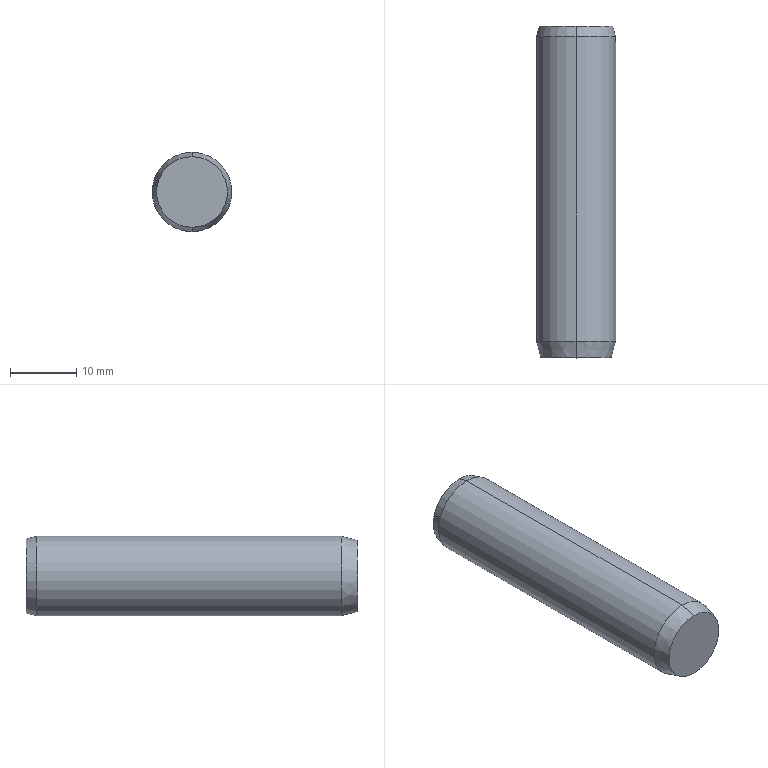Part | SolidWorks | features Chamfer 2, Extrusion 1, HoleWzd 1 | 1 solid | 12 faces | box 12 x 50 x 12 mm | volume 5242 mm3 | cone 6 | cylinder 4 | plane 2 | commonest cylinder face diameters 4.8 x2 12 x2
STEP:
#1=CARTESIAN_POINT('',(0.,-25.,-5.33));
#2=VERTEX_POINT('',#1);
#3=CARTESIAN_POINT('',(0.,-25.,5.33));
#4=VERTEX_POINT('',#3);
#5=CARTESIAN_POINT('',(0.,-25.,0.));
#6=DIRECTION('',(0.,-1.,0.));
#7=DIRECTION('',(0.,0.,1.));
#8=AXIS2_PLACEMENT_3D('',#5,#6,#7);
#9=CIRCLE('',#8,5.33);
#10=EDGE_CURVE('',#2,#4,#9,.T.);
#11=ORIENTED_EDGE('',*,*,#10,.F.);
#12=CARTESIAN_POINT('',(0.,-22.5,-6.));
#13=VERTEX_POINT('',#12);
#14=CARTESIAN_POINT('',(0.,-22.5,-6.));
#15=DIRECTION('',(0.,0.9659,-0.2588));
#16=VECTOR('',#15,1000.);
#17=LINE('',#14,#16);
#18=EDGE_CURVE('',#2,#13,#17,.T.);
#19=ORIENTED_EDGE('',*,*,#18,.T.);
#20=CARTESIAN_POINT('',(0.,-22.5,6.));
#21=VERTEX_POINT('',#20);
#22=CARTESIAN_POINT('',(0.,-22.5,0.));
#23=DIRECTION('',(0.,1.,0.));
#24=DIRECTION('',(0.,0.,1.));
#25=AXIS2_PLACEMENT_3D('',#22,#23,#24);
#26=CIRCLE('',#25,6.);
#27=EDGE_CURVE('',#21,#13,#26,.T.);
#28=ORIENTED_EDGE('',*,*,#27,.F.);
#29=CARTESIAN_POINT('',(0.,-22.5,6.));
#30=DIRECTION('',(0.,0.9659,0.2588));
#31=VECTOR('',#30,1000.);
#32=LINE('',#29,#31);
#33=EDGE_CURVE('',#4,#21,#32,.T.);
#34=ORIENTED_EDGE('',*,*,#33,.F.);
#35=EDGE_LOOP('',(#11,#19,#28,#34));
#36=FACE_OUTER_BOUND('',#35,.T.);
#37=CARTESIAN_POINT('',(0.,-22.5,0.));
#38=DIRECTION('',(0.,1.,0.));
#39=DIRECTION('',(0.,0.,1.));
#40=AXIS2_PLACEMENT_3D('',#37,#38,#39);
#41=CONICAL_SURFACE('',#40,6.,0.2618);
#42=ADVANCED_FACE('',(#36),#41,.T.);
#43=CARTESIAN_POINT('',(0.,25.,5.571));
#44=VERTEX_POINT('',#43);
#45=CARTESIAN_POINT('',(0.,25.,-5.571));
#46=VERTEX_POINT('',#45);
#47=CARTESIAN_POINT('',(0.,25.,0.));
#48=DIRECTION('',(0.,1.,0.));
#49=DIRECTION('',(0.,0.,1.));
#50=AXIS2_PLACEMENT_3D('',#47,#48,#49);
#51=CIRCLE('',#50,5.571);
#52=EDGE_CURVE('',#44,#46,#51,.T.);
#53=ORIENTED_EDGE('',*,*,#52,.F.);
#54=CARTESIAN_POINT('',(0.,23.4,6.));
#55=VERTEX_POINT('',#54);
#56=CARTESIAN_POINT('',(0.,25.,5.571));
#57=DIRECTION('',(0.,-0.9659,0.2588));
#58=VECTOR('',#57,1000.);
#59=LINE('',#56,#58);
#60=EDGE_CURVE('',#44,#55,#59,.T.);
#61=ORIENTED_EDGE('',*,*,#60,.T.);
#62=CARTESIAN_POINT('',(0.,23.4,-6.));
#63=VERTEX_POINT('',#62);
#64=CARTESIAN_POINT('',(0.,23.4,0.));
#65=DIRECTION('',(0.,-1.,0.));
#66=DIRECTION('',(0.,0.,1.));
#67=AXIS2_PLACEMENT_3D('',#64,#65,#66);
#68=CIRCLE('',#67,6.);
#69=EDGE_CURVE('',#63,#55,#68,.T.);
#70=ORIENTED_EDGE('',*,*,#69,.F.);
#71=CARTESIAN_POINT('',(0.,25.,-5.571));
#72=DIRECTION('',(0.,-0.9659,-0.2588));
#73=VECTOR('',#72,1000.);
#74=LINE('',#71,#73);
#75=EDGE_CURVE('',#46,#63,#74,.T.);
#76=ORIENTED_EDGE('',*,*,#75,.F.);
#77=EDGE_LOOP('',(#53,#61,#70,#76));
#78=FACE_OUTER_BOUND('',#77,.T.);
#79=CARTESIAN_POINT('',(0.,25.,0.));
#80=DIRECTION('',(0.,-1.,0.));
#81=DIRECTION('',(0.,0.,-1.));
#82=AXIS2_PLACEMENT_3D('',#79,#80,#81);
#83=CONICAL_SURFACE('',#82,5.571,0.2618);
#84=ADVANCED_FACE('',(#78),#83,.T.);
#85=CARTESIAN_POINT('',(0.,5.,-2.4));
#86=VERTEX_POINT('',#85);
#87=CARTESIAN_POINT('',(0.,5.,2.4));
#88=VERTEX_POINT('',#87);
#89=CARTESIAN_POINT('',(0.,5.,0.));
#90=DIRECTION('',(0.,1.,0.));
#91=DIRECTION('',(0.,0.,1.));
#92=AXIS2_PLACEMENT_3D('',#89,#90,#91);
#93=CIRCLE('',#92,2.4);
#94=EDGE_CURVE('',#86,#88,#93,.T.);
#95=ORIENTED_EDGE('',*,*,#94,.F.);
#96=CARTESIAN_POINT('',(0.,25.,-2.4));
#97=VERTEX_POINT('',#96);
#98=CARTESIAN_POINT('',(0.,25.,-2.4));
#99=DIRECTION('',(0.,1.,0.));
#100=VECTOR('',#99,1000.);
#101=LINE('',#98,#100);
#102=EDGE_CURVE('',#86,#97,#101,.T.);
#103=ORIENTED_EDGE('',*,*,#102,.T.);
#104=CARTESIAN_POINT('',(0.,25.,2.4));
#105=VERTEX_POINT('',#104);
#106=CARTESIAN_POINT('',(0.,25.,0.));
#107=DIRECTION('',(0.,1.,0.));
#108=DIRECTION('',(0.,0.,1.));
#109=AXIS2_PLACEMENT_3D('',#106,#107,#108);
#110=CIRCLE('',#109,2.4);
#111=EDGE_CURVE('',#97,#105,#110,.T.);
#112=ORIENTED_EDGE('',*,*,#111,.T.);
#113=CARTESIAN_POINT('',(0.,25.,2.4));
#114=DIRECTION('',(0.,1.,0.));
#115=VECTOR('',#114,1000.);
#116=LINE('',#113,#115);
#117=EDGE_CURVE('',#88,#105,#116,.T.);
#118=ORIENTED_EDGE('',*,*,#117,.F.);
#119=EDGE_LOOP('',(#95,#103,#112,#118));
#120=FACE_OUTER_BOUND('',#119,.T.);
#121=CARTESIAN_POINT('',(0.,25.,0.));
#122=DIRECTION('',(0.,1.,0.));
#123=DIRECTION('',(0.,0.,1.));
#124=AXIS2_PLACEMENT_3D('',#121,#122,#123);
#125=CYLINDRICAL_SURFACE('',#124,2.4);
#126=ADVANCED_FACE('',(#120),#125,.F.);
#127=CARTESIAN_POINT('',(0.,3.614,0.));
#128=VERTEX_POINT('',#127);
#129=CARTESIAN_POINT('',(0.,5.,2.4));
#130=DIRECTION('',(0.,0.5,0.866));
#131=VECTOR('',#130,1000.);
#132=LINE('',#129,#131);
#133=EDGE_CURVE('',#128,#88,#132,.T.);
#134=ORIENTED_EDGE('',*,*,#133,.F.);
#135=CARTESIAN_POINT('',(0.,5.,-2.4));
#136=DIRECTION('',(0.,0.5,-0.866));
#137=VECTOR('',#136,1000.);
#138=LINE('',#135,#137);
#139=EDGE_CURVE('',#128,#86,#138,.T.);
#140=ORIENTED_EDGE('',*,*,#139,.T.);
#141=ORIENTED_EDGE('',*,*,#94,.T.);
#142=EDGE_LOOP('',(#134,#140,#141));
#143=FACE_OUTER_BOUND('',#142,.T.);
#144=CARTESIAN_POINT('',(0.,5.,0.));
#145=DIRECTION('',(0.,1.,0.));
#146=DIRECTION('',(0.,0.,1.));
#147=AXIS2_PLACEMENT_3D('',#144,#145,#146);
#148=CONICAL_SURFACE('',#147,2.4,1.047);
#149=ADVANCED_FACE('',(#143),#148,.F.);
#150=ORIENTED_EDGE('',*,*,#69,.T.);
#151=CARTESIAN_POINT('',(0.,25.,6.));
#152=DIRECTION('',(0.,-1.,0.));
#153=VECTOR('',#152,1000.);
#154=LINE('',#151,#153);
#155=EDGE_CURVE('',#55,#21,#154,.T.);
#156=ORIENTED_EDGE('',*,*,#155,.T.);
#157=ORIENTED_EDGE('',*,*,#27,.T.);
#158=CARTESIAN_POINT('',(0.,25.,-6.));
#159=DIRECTION('',(0.,-1.,0.));
#160=VECTOR('',#159,1000.);
#161=LINE('',#158,#160);
#162=EDGE_CURVE('',#63,#13,#161,.T.);
#163=ORIENTED_EDGE('',*,*,#162,.F.);
#164=EDGE_LOOP('',(#150,#156,#157,#163));
#165=FACE_OUTER_BOUND('',#164,.T.);
#166=CARTESIAN_POINT('',(0.,25.,0.));
#167=DIRECTION('',(0.,-1.,0.));
#168=DIRECTION('',(0.,0.,-1.));
#169=AXIS2_PLACEMENT_3D('',#166,#167,#168);
#170=CYLINDRICAL_SURFACE('',#169,6.);
#171=ADVANCED_FACE('',(#165),#170,.T.);
#172=ORIENTED_EDGE('',*,*,#155,.F.);
#173=CARTESIAN_POINT('',(0.,23.4,0.));
#174=DIRECTION('',(0.,-1.,0.));
#175=DIRECTION('',(0.,0.,1.));
#176=AXIS2_PLACEMENT_3D('',#173,#174,#175);
#177=CIRCLE('',#176,6.);
#178=EDGE_CURVE('',#55,#63,#177,.T.);
#179=ORIENTED_EDGE('',*,*,#178,.T.);
#180=ORIENTED_EDGE('',*,*,#162,.T.);
#181=CARTESIAN_POINT('',(0.,-22.5,0.));
#182=DIRECTION('',(0.,1.,0.));
#183=DIRECTION('',(0.,0.,1.));
#184=AXIS2_PLACEMENT_3D('',#181,#182,#183);
#185=CIRCLE('',#184,6.);
#186=EDGE_CURVE('',#13,#21,#185,.T.);
#187=ORIENTED_EDGE('',*,*,#186,.T.);
#188=EDGE_LOOP('',(#172,#179,#180,#187));
#189=FACE_OUTER_BOUND('',#188,.T.);
#190=CARTESIAN_POINT('',(0.,25.,0.));
#191=DIRECTION('',(0.,-1.,0.));
#192=DIRECTION('',(0.,0.,-1.));
#193=AXIS2_PLACEMENT_3D('',#190,#191,#192);
#194=CYLINDRICAL_SURFACE('',#193,6.);
#195=ADVANCED_FACE('',(#189),#194,.T.);
#196=CARTESIAN_POINT('',(0.,25.,0.));
#197=DIRECTION('',(0.,1.,0.));
#198=DIRECTION('',(0.,0.,1.));
#199=AXIS2_PLACEMENT_3D('',#196,#197,#198);
#200=CIRCLE('',#199,5.571);
#201=EDGE_CURVE('',#46,#44,#200,.T.);
#202=ORIENTED_EDGE('',*,*,#201,.T.);
#203=ORIENTED_EDGE('',*,*,#52,.T.);
#204=EDGE_LOOP('',(#202,#203));
#205=FACE_OUTER_BOUND('',#204,.T.);
#206=CARTESIAN_POINT('',(0.,25.,0.));
#207=DIRECTION('',(0.,1.,0.));
#208=DIRECTION('',(0.,0.,1.));
#209=AXIS2_PLACEMENT_3D('',#206,#207,#208);
#210=CIRCLE('',#209,2.4);
#211=EDGE_CURVE('',#105,#97,#210,.T.);
#212=ORIENTED_EDGE('',*,*,#211,.F.);
#213=ORIENTED_EDGE('',*,*,#111,.F.);
#214=EDGE_LOOP('',(#212,#213));
#215=FACE_BOUND('',#214,.T.);
#216=CARTESIAN_POINT('',(0.,25.,0.));
#217=DIRECTION('',(0.,1.,0.));
#218=DIRECTION('',(0.,0.,1.));
#219=AXIS2_PLACEMENT_3D('',#216,#217,#218);
#220=PLANE('',#219);
#221=ADVANCED_FACE('',(#205,#215),#220,.T.);
#222=CARTESIAN_POINT('',(0.,-25.,0.));
#223=DIRECTION('',(0.,-1.,0.));
#224=DIRECTION('',(0.,0.,1.));
#225=AXIS2_PLACEMENT_3D('',#222,#223,#224);
#226=CIRCLE('',#225,5.33);
#227=EDGE_CURVE('',#4,#2,#226,.T.);
#228=ORIENTED_EDGE('',*,*,#227,.T.);
#229=ORIENTED_EDGE('',*,*,#10,.T.);
#230=EDGE_LOOP('',(#228,#229));
#231=FACE_OUTER_BOUND('',#230,.T.);
#232=CARTESIAN_POINT('',(0.,-25.,0.));
#233=DIRECTION('',(0.,1.,0.));
#234=DIRECTION('',(0.,0.,1.));
#235=AXIS2_PLACEMENT_3D('',#232,#233,#234);
#236=PLANE('',#235);
#237=ADVANCED_FACE('',(#231),#236,.F.);
#238=ORIENTED_EDGE('',*,*,#139,.F.);
#239=ORIENTED_EDGE('',*,*,#133,.T.);
#240=CARTESIAN_POINT('',(0.,5.,0.));
#241=DIRECTION('',(0.,1.,0.));
#242=DIRECTION('',(0.,0.,1.));
#243=AXIS2_PLACEMENT_3D('',#240,#241,#242);
#244=CIRCLE('',#243,2.4);
#245=EDGE_CURVE('',#88,#86,#244,.T.);
#246=ORIENTED_EDGE('',*,*,#245,.T.);
#247=EDGE_LOOP('',(#238,#239,#246));
#248=FACE_OUTER_BOUND('',#247,.T.);
#249=CARTESIAN_POINT('',(0.,5.,0.));
#250=DIRECTION('',(0.,1.,0.));
#251=DIRECTION('',(0.,0.,1.));
#252=AXIS2_PLACEMENT_3D('',#249,#250,#251);
#253=CONICAL_SURFACE('',#252,2.4,1.047);
#254=ADVANCED_FACE('',(#248),#253,.F.);
#255=ORIENTED_EDGE('',*,*,#102,.F.);
#256=ORIENTED_EDGE('',*,*,#245,.F.);
#257=ORIENTED_EDGE('',*,*,#117,.T.);
#258=ORIENTED_EDGE('',*,*,#211,.T.);
#259=EDGE_LOOP('',(#255,#256,#257,#258));
#260=FACE_OUTER_BOUND('',#259,.T.);
#261=CARTESIAN_POINT('',(0.,25.,0.));
#262=DIRECTION('',(0.,1.,0.));
#263=DIRECTION('',(0.,0.,1.));
#264=AXIS2_PLACEMENT_3D('',#261,#262,#263);
#265=CYLINDRICAL_SURFACE('',#264,2.4);
#266=ADVANCED_FACE('',(#260),#265,.F.);
#267=ORIENTED_EDGE('',*,*,#60,.F.);
#268=ORIENTED_EDGE('',*,*,#201,.F.);
#269=ORIENTED_EDGE('',*,*,#75,.T.);
#270=ORIENTED_EDGE('',*,*,#178,.F.);
#271=EDGE_LOOP('',(#267,#268,#269,#270));
#272=FACE_OUTER_BOUND('',#271,.T.);
#273=CARTESIAN_POINT('',(0.,25.,0.));
#274=DIRECTION('',(0.,-1.,0.));
#275=DIRECTION('',(0.,0.,-1.));
#276=AXIS2_PLACEMENT_3D('',#273,#274,#275);
#277=CONICAL_SURFACE('',#276,5.571,0.2618);
#278=ADVANCED_FACE('',(#272),#277,.T.);
#279=ORIENTED_EDGE('',*,*,#18,.F.);
#280=ORIENTED_EDGE('',*,*,#227,.F.);
#281=ORIENTED_EDGE('',*,*,#33,.T.);
#282=ORIENTED_EDGE('',*,*,#186,.F.);
#283=EDGE_LOOP('',(#279,#280,#281,#282));
#284=FACE_OUTER_BOUND('',#283,.T.);
#285=CARTESIAN_POINT('',(0.,-22.5,0.));
#286=DIRECTION('',(0.,1.,0.));
#287=DIRECTION('',(0.,0.,1.));
#288=AXIS2_PLACEMENT_3D('',#285,#286,#287);
#289=CONICAL_SURFACE('',#288,6.,0.2618);
#290=ADVANCED_FACE('',(#284),#289,.T.);
#291=CLOSED_SHELL('',(#42,#84,#126,#149,#171,#195,#221,#237,#254,#266,#278,#290));
#292=MANIFOLD_SOLID_BREP('',#291);
#293=CARTESIAN_POINT('',(0.,0.,0.));
#294=DIRECTION('',(0.,0.,1.));
#295=DIRECTION('',(1.,0.,0.));
#296=AXIS2_PLACEMENT_3D('',#293,#294,#295);
#297=(LENGTH_UNIT()NAMED_UNIT(*)SI_UNIT(.MILLI.,.METRE.));
#298=UNCERTAINTY_MEASURE_WITH_UNIT(LENGTH_MEASURE(0.00001),#297,'','');
#299=(NAMED_UNIT(*)PLANE_ANGLE_UNIT()SI_UNIT($,.RADIAN.));
#300=(NAMED_UNIT(*)SI_UNIT($,.STERADIAN.)SOLID_ANGLE_UNIT());
#301=(GEOMETRIC_REPRESENTATION_CONTEXT(3)GLOBAL_UNCERTAINTY_ASSIGNED_CONTEXT((#298))GLOBAL_UNIT_ASSIGNED_CONTEXT((#297,#299,#300))REPRESENTATION_CONTEXT('',''));
#302=ADVANCED_BREP_SHAPE_REPRESENTATION('',(#292,#296),#301);